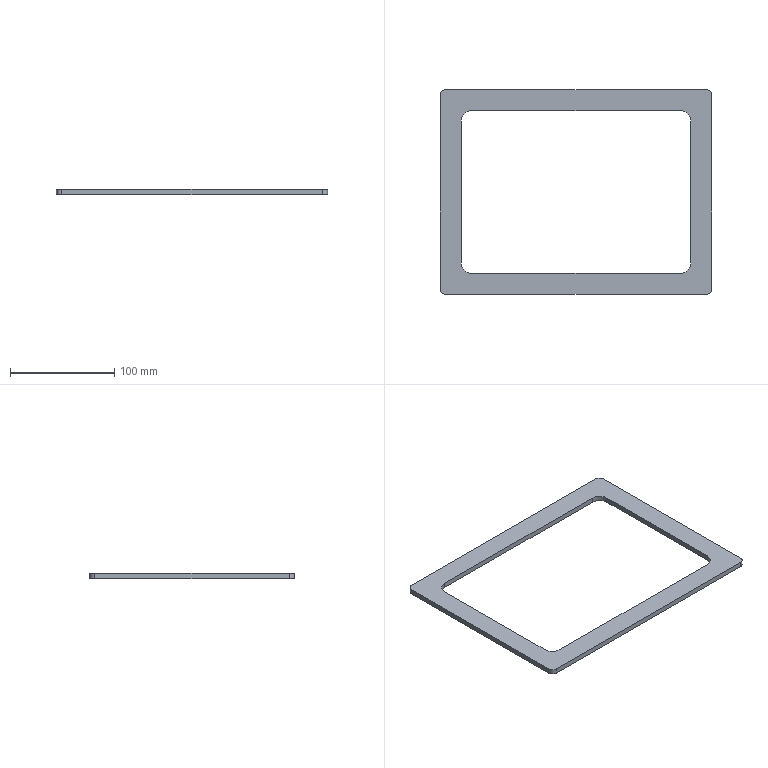Part | SolidWorks | features Fillet 2, Extrusion 1 | 1 solid | 18 faces | box 260 x 196 x 5 mm | volume 83522 mm3 | plane 10 | cylinder 8 | commonest cylinder face diameters 10 x4 20 x4
STEP:
#1=CARTESIAN_POINT('',(130.,-93.,5.));
#2=VERTEX_POINT('',#1);
#3=CARTESIAN_POINT('',(130.,93.,5.));
#4=VERTEX_POINT('',#3);
#5=CARTESIAN_POINT('',(130.,98.,5.));
#6=DIRECTION('',(0.,1.,0.));
#7=VECTOR('',#6,1000.);
#8=LINE('',#5,#7);
#9=EDGE_CURVE('',#2,#4,#8,.T.);
#10=ORIENTED_EDGE('',*,*,#9,.T.);
#11=CARTESIAN_POINT('',(125.,98.,5.));
#12=VERTEX_POINT('',#11);
#13=CARTESIAN_POINT('',(125.,93.,5.));
#14=DIRECTION('',(0.,0.,1.));
#15=DIRECTION('',(1.,0.,0.));
#16=AXIS2_PLACEMENT_3D('',#13,#14,#15);
#17=CIRCLE('',#16,5.);
#18=EDGE_CURVE('',#4,#12,#17,.T.);
#19=ORIENTED_EDGE('',*,*,#18,.T.);
#20=CARTESIAN_POINT('',(-125.,98.,5.));
#21=VERTEX_POINT('',#20);
#22=CARTESIAN_POINT('',(-130.,98.,5.));
#23=DIRECTION('',(-1.,0.,0.));
#24=VECTOR('',#23,1000.);
#25=LINE('',#22,#24);
#26=EDGE_CURVE('',#12,#21,#25,.T.);
#27=ORIENTED_EDGE('',*,*,#26,.T.);
#28=CARTESIAN_POINT('',(-130.,93.,5.));
#29=VERTEX_POINT('',#28);
#30=CARTESIAN_POINT('',(-125.,93.,5.));
#31=DIRECTION('',(0.,0.,1.));
#32=DIRECTION('',(1.,0.,0.));
#33=AXIS2_PLACEMENT_3D('',#30,#31,#32);
#34=CIRCLE('',#33,5.);
#35=EDGE_CURVE('',#21,#29,#34,.T.);
#36=ORIENTED_EDGE('',*,*,#35,.T.);
#37=CARTESIAN_POINT('',(-130.,-93.,5.));
#38=VERTEX_POINT('',#37);
#39=CARTESIAN_POINT('',(-130.,98.,5.));
#40=DIRECTION('',(0.,-1.,0.));
#41=VECTOR('',#40,1000.);
#42=LINE('',#39,#41);
#43=EDGE_CURVE('',#29,#38,#42,.T.);
#44=ORIENTED_EDGE('',*,*,#43,.T.);
#45=CARTESIAN_POINT('',(-125.,-98.,5.));
#46=VERTEX_POINT('',#45);
#47=CARTESIAN_POINT('',(-125.,-93.,5.));
#48=DIRECTION('',(0.,0.,1.));
#49=DIRECTION('',(1.,0.,0.));
#50=AXIS2_PLACEMENT_3D('',#47,#48,#49);
#51=CIRCLE('',#50,5.);
#52=EDGE_CURVE('',#38,#46,#51,.T.);
#53=ORIENTED_EDGE('',*,*,#52,.T.);
#54=CARTESIAN_POINT('',(125.,-98.,5.));
#55=VERTEX_POINT('',#54);
#56=CARTESIAN_POINT('',(-130.,-98.,5.));
#57=DIRECTION('',(1.,0.,0.));
#58=VECTOR('',#57,1000.);
#59=LINE('',#56,#58);
#60=EDGE_CURVE('',#46,#55,#59,.T.);
#61=ORIENTED_EDGE('',*,*,#60,.T.);
#62=CARTESIAN_POINT('',(125.,-93.,5.));
#63=DIRECTION('',(0.,0.,1.));
#64=DIRECTION('',(1.,0.,0.));
#65=AXIS2_PLACEMENT_3D('',#62,#63,#64);
#66=CIRCLE('',#65,5.);
#67=EDGE_CURVE('',#55,#2,#66,.T.);
#68=ORIENTED_EDGE('',*,*,#67,.T.);
#69=EDGE_LOOP('',(#10,#19,#27,#36,#44,#53,#61,#68));
#70=FACE_OUTER_BOUND('',#69,.T.);
#71=CARTESIAN_POINT('',(-100.,-78.,5.));
#72=VERTEX_POINT('',#71);
#73=CARTESIAN_POINT('',(100.,-78.,5.));
#74=VERTEX_POINT('',#73);
#75=CARTESIAN_POINT('',(-110.,-78.,5.));
#76=DIRECTION('',(1.,0.,0.));
#77=VECTOR('',#76,1000.);
#78=LINE('',#75,#77);
#79=EDGE_CURVE('',#72,#74,#78,.T.);
#80=ORIENTED_EDGE('',*,*,#79,.F.);
#81=CARTESIAN_POINT('',(-110.,-68.,5.));
#82=VERTEX_POINT('',#81);
#83=CARTESIAN_POINT('',(-100.,-68.,5.));
#84=DIRECTION('',(0.,0.,-1.));
#85=DIRECTION('',(1.,0.,0.));
#86=AXIS2_PLACEMENT_3D('',#83,#84,#85);
#87=CIRCLE('',#86,10.);
#88=EDGE_CURVE('',#72,#82,#87,.T.);
#89=ORIENTED_EDGE('',*,*,#88,.T.);
#90=CARTESIAN_POINT('',(-110.,68.,5.));
#91=VERTEX_POINT('',#90);
#92=CARTESIAN_POINT('',(-110.,78.,5.));
#93=DIRECTION('',(0.,-1.,0.));
#94=VECTOR('',#93,1000.);
#95=LINE('',#92,#94);
#96=EDGE_CURVE('',#91,#82,#95,.T.);
#97=ORIENTED_EDGE('',*,*,#96,.F.);
#98=CARTESIAN_POINT('',(-100.,78.,5.));
#99=VERTEX_POINT('',#98);
#100=CARTESIAN_POINT('',(-100.,68.,5.));
#101=DIRECTION('',(0.,0.,-1.));
#102=DIRECTION('',(1.,0.,0.));
#103=AXIS2_PLACEMENT_3D('',#100,#101,#102);
#104=CIRCLE('',#103,10.);
#105=EDGE_CURVE('',#91,#99,#104,.T.);
#106=ORIENTED_EDGE('',*,*,#105,.T.);
#107=CARTESIAN_POINT('',(100.,78.,5.));
#108=VERTEX_POINT('',#107);
#109=CARTESIAN_POINT('',(-110.,78.,5.));
#110=DIRECTION('',(-1.,0.,0.));
#111=VECTOR('',#110,1000.);
#112=LINE('',#109,#111);
#113=EDGE_CURVE('',#108,#99,#112,.T.);
#114=ORIENTED_EDGE('',*,*,#113,.F.);
#115=CARTESIAN_POINT('',(110.,68.,5.));
#116=VERTEX_POINT('',#115);
#117=CARTESIAN_POINT('',(100.,68.,5.));
#118=DIRECTION('',(0.,0.,-1.));
#119=DIRECTION('',(1.,0.,0.));
#120=AXIS2_PLACEMENT_3D('',#117,#118,#119);
#121=CIRCLE('',#120,10.);
#122=EDGE_CURVE('',#108,#116,#121,.T.);
#123=ORIENTED_EDGE('',*,*,#122,.T.);
#124=CARTESIAN_POINT('',(110.,-68.,5.));
#125=VERTEX_POINT('',#124);
#126=CARTESIAN_POINT('',(110.,78.,5.));
#127=DIRECTION('',(0.,1.,0.));
#128=VECTOR('',#127,1000.);
#129=LINE('',#126,#128);
#130=EDGE_CURVE('',#125,#116,#129,.T.);
#131=ORIENTED_EDGE('',*,*,#130,.F.);
#132=CARTESIAN_POINT('',(100.,-68.,5.));
#133=DIRECTION('',(0.,0.,-1.));
#134=DIRECTION('',(1.,0.,0.));
#135=AXIS2_PLACEMENT_3D('',#132,#133,#134);
#136=CIRCLE('',#135,10.);
#137=EDGE_CURVE('',#125,#74,#136,.T.);
#138=ORIENTED_EDGE('',*,*,#137,.T.);
#139=EDGE_LOOP('',(#80,#89,#97,#106,#114,#123,#131,#138));
#140=FACE_BOUND('',#139,.T.);
#141=CARTESIAN_POINT('',(0.,0.,5.));
#142=DIRECTION('',(0.,0.,1.));
#143=DIRECTION('',(1.,0.,0.));
#144=AXIS2_PLACEMENT_3D('',#141,#142,#143);
#145=PLANE('',#144);
#146=ADVANCED_FACE('',(#70,#140),#145,.T.);
#147=CARTESIAN_POINT('',(125.,98.,0.));
#148=VERTEX_POINT('',#147);
#149=CARTESIAN_POINT('',(-125.,98.,0.));
#150=VERTEX_POINT('',#149);
#151=CARTESIAN_POINT('',(-130.,98.,0.));
#152=DIRECTION('',(-1.,0.,0.));
#153=VECTOR('',#152,1000.);
#154=LINE('',#151,#153);
#155=EDGE_CURVE('',#148,#150,#154,.T.);
#156=ORIENTED_EDGE('',*,*,#155,.F.);
#157=CARTESIAN_POINT('',(130.,93.,0.));
#158=VERTEX_POINT('',#157);
#159=CARTESIAN_POINT('',(125.,93.,0.));
#160=DIRECTION('',(0.,0.,-1.));
#161=DIRECTION('',(1.,0.,0.));
#162=AXIS2_PLACEMENT_3D('',#159,#160,#161);
#163=CIRCLE('',#162,5.);
#164=EDGE_CURVE('',#148,#158,#163,.T.);
#165=ORIENTED_EDGE('',*,*,#164,.T.);
#166=CARTESIAN_POINT('',(130.,-93.,0.));
#167=VERTEX_POINT('',#166);
#168=CARTESIAN_POINT('',(130.,98.,0.));
#169=DIRECTION('',(0.,1.,0.));
#170=VECTOR('',#169,1000.);
#171=LINE('',#168,#170);
#172=EDGE_CURVE('',#167,#158,#171,.T.);
#173=ORIENTED_EDGE('',*,*,#172,.F.);
#174=CARTESIAN_POINT('',(125.,-98.,0.));
#175=VERTEX_POINT('',#174);
#176=CARTESIAN_POINT('',(125.,-93.,0.));
#177=DIRECTION('',(0.,0.,-1.));
#178=DIRECTION('',(1.,0.,0.));
#179=AXIS2_PLACEMENT_3D('',#176,#177,#178);
#180=CIRCLE('',#179,5.);
#181=EDGE_CURVE('',#167,#175,#180,.T.);
#182=ORIENTED_EDGE('',*,*,#181,.T.);
#183=CARTESIAN_POINT('',(-125.,-98.,0.));
#184=VERTEX_POINT('',#183);
#185=CARTESIAN_POINT('',(-130.,-98.,0.));
#186=DIRECTION('',(1.,0.,0.));
#187=VECTOR('',#186,1000.);
#188=LINE('',#185,#187);
#189=EDGE_CURVE('',#184,#175,#188,.T.);
#190=ORIENTED_EDGE('',*,*,#189,.F.);
#191=CARTESIAN_POINT('',(-130.,-93.,0.));
#192=VERTEX_POINT('',#191);
#193=CARTESIAN_POINT('',(-125.,-93.,0.));
#194=DIRECTION('',(0.,0.,-1.));
#195=DIRECTION('',(1.,0.,0.));
#196=AXIS2_PLACEMENT_3D('',#193,#194,#195);
#197=CIRCLE('',#196,5.);
#198=EDGE_CURVE('',#184,#192,#197,.T.);
#199=ORIENTED_EDGE('',*,*,#198,.T.);
#200=CARTESIAN_POINT('',(-130.,93.,0.));
#201=VERTEX_POINT('',#200);
#202=CARTESIAN_POINT('',(-130.,98.,0.));
#203=DIRECTION('',(0.,-1.,0.));
#204=VECTOR('',#203,1000.);
#205=LINE('',#202,#204);
#206=EDGE_CURVE('',#201,#192,#205,.T.);
#207=ORIENTED_EDGE('',*,*,#206,.F.);
#208=CARTESIAN_POINT('',(-125.,93.,0.));
#209=DIRECTION('',(0.,0.,-1.));
#210=DIRECTION('',(1.,0.,0.));
#211=AXIS2_PLACEMENT_3D('',#208,#209,#210);
#212=CIRCLE('',#211,5.);
#213=EDGE_CURVE('',#201,#150,#212,.T.);
#214=ORIENTED_EDGE('',*,*,#213,.T.);
#215=EDGE_LOOP('',(#156,#165,#173,#182,#190,#199,#207,#214));
#216=FACE_OUTER_BOUND('',#215,.T.);
#217=CARTESIAN_POINT('',(100.,78.,0.));
#218=VERTEX_POINT('',#217);
#219=CARTESIAN_POINT('',(-100.,78.,0.));
#220=VERTEX_POINT('',#219);
#221=CARTESIAN_POINT('',(-110.,78.,0.));
#222=DIRECTION('',(-1.,0.,0.));
#223=VECTOR('',#222,1000.);
#224=LINE('',#221,#223);
#225=EDGE_CURVE('',#218,#220,#224,.T.);
#226=ORIENTED_EDGE('',*,*,#225,.T.);
#227=CARTESIAN_POINT('',(-110.,68.,0.));
#228=VERTEX_POINT('',#227);
#229=CARTESIAN_POINT('',(-100.,68.,0.));
#230=DIRECTION('',(0.,0.,1.));
#231=DIRECTION('',(1.,0.,0.));
#232=AXIS2_PLACEMENT_3D('',#229,#230,#231);
#233=CIRCLE('',#232,10.);
#234=EDGE_CURVE('',#220,#228,#233,.T.);
#235=ORIENTED_EDGE('',*,*,#234,.T.);
#236=CARTESIAN_POINT('',(-110.,-68.,0.));
#237=VERTEX_POINT('',#236);
#238=CARTESIAN_POINT('',(-110.,78.,0.));
#239=DIRECTION('',(0.,-1.,0.));
#240=VECTOR('',#239,1000.);
#241=LINE('',#238,#240);
#242=EDGE_CURVE('',#228,#237,#241,.T.);
#243=ORIENTED_EDGE('',*,*,#242,.T.);
#244=CARTESIAN_POINT('',(-100.,-78.,0.));
#245=VERTEX_POINT('',#244);
#246=CARTESIAN_POINT('',(-100.,-68.,0.));
#247=DIRECTION('',(0.,0.,1.));
#248=DIRECTION('',(1.,0.,0.));
#249=AXIS2_PLACEMENT_3D('',#246,#247,#248);
#250=CIRCLE('',#249,10.);
#251=EDGE_CURVE('',#237,#245,#250,.T.);
#252=ORIENTED_EDGE('',*,*,#251,.T.);
#253=CARTESIAN_POINT('',(100.,-78.,0.));
#254=VERTEX_POINT('',#253);
#255=CARTESIAN_POINT('',(-110.,-78.,0.));
#256=DIRECTION('',(1.,0.,0.));
#257=VECTOR('',#256,1000.);
#258=LINE('',#255,#257);
#259=EDGE_CURVE('',#245,#254,#258,.T.);
#260=ORIENTED_EDGE('',*,*,#259,.T.);
#261=CARTESIAN_POINT('',(110.,-68.,0.));
#262=VERTEX_POINT('',#261);
#263=CARTESIAN_POINT('',(100.,-68.,0.));
#264=DIRECTION('',(0.,0.,1.));
#265=DIRECTION('',(1.,0.,0.));
#266=AXIS2_PLACEMENT_3D('',#263,#264,#265);
#267=CIRCLE('',#266,10.);
#268=EDGE_CURVE('',#254,#262,#267,.T.);
#269=ORIENTED_EDGE('',*,*,#268,.T.);
#270=CARTESIAN_POINT('',(110.,68.,0.));
#271=VERTEX_POINT('',#270);
#272=CARTESIAN_POINT('',(110.,78.,0.));
#273=DIRECTION('',(0.,1.,0.));
#274=VECTOR('',#273,1000.);
#275=LINE('',#272,#274);
#276=EDGE_CURVE('',#262,#271,#275,.T.);
#277=ORIENTED_EDGE('',*,*,#276,.T.);
#278=CARTESIAN_POINT('',(100.,68.,0.));
#279=DIRECTION('',(0.,0.,1.));
#280=DIRECTION('',(1.,0.,0.));
#281=AXIS2_PLACEMENT_3D('',#278,#279,#280);
#282=CIRCLE('',#281,10.);
#283=EDGE_CURVE('',#271,#218,#282,.T.);
#284=ORIENTED_EDGE('',*,*,#283,.T.);
#285=EDGE_LOOP('',(#226,#235,#243,#252,#260,#269,#277,#284));
#286=FACE_BOUND('',#285,.T.);
#287=CARTESIAN_POINT('',(0.,0.,0.));
#288=DIRECTION('',(0.,0.,1.));
#289=DIRECTION('',(1.,0.,0.));
#290=AXIS2_PLACEMENT_3D('',#287,#288,#289);
#291=PLANE('',#290);
#292=ADVANCED_FACE('',(#216,#286),#291,.F.);
#293=ORIENTED_EDGE('',*,*,#206,.T.);
#294=CARTESIAN_POINT('',(-130.,-93.,5.));
#295=DIRECTION('',(0.,0.,1.));
#296=VECTOR('',#295,1000.);
#297=LINE('',#294,#296);
#298=EDGE_CURVE('',#192,#38,#297,.T.);
#299=ORIENTED_EDGE('',*,*,#298,.T.);
#300=ORIENTED_EDGE('',*,*,#43,.F.);
#301=CARTESIAN_POINT('',(-130.,93.,5.));
#302=DIRECTION('',(0.,0.,-1.));
#303=VECTOR('',#302,1000.);
#304=LINE('',#301,#303);
#305=EDGE_CURVE('',#29,#201,#304,.T.);
#306=ORIENTED_EDGE('',*,*,#305,.T.);
#307=EDGE_LOOP('',(#293,#299,#300,#306));
#308=FACE_OUTER_BOUND('',#307,.T.);
#309=CARTESIAN_POINT('',(-130.,98.,5.));
#310=DIRECTION('',(1.,0.,0.));
#311=DIRECTION('',(0.,0.,-1.));
#312=AXIS2_PLACEMENT_3D('',#309,#310,#311);
#313=PLANE('',#312);
#314=ADVANCED_FACE('',(#308),#313,.F.);
#315=ORIENTED_EDGE('',*,*,#189,.T.);
#316=CARTESIAN_POINT('',(125.,-98.,5.));
#317=DIRECTION('',(0.,0.,1.));
#318=VECTOR('',#317,1000.);
#319=LINE('',#316,#318);
#320=EDGE_CURVE('',#175,#55,#319,.T.);
#321=ORIENTED_EDGE('',*,*,#320,.T.);
#322=ORIENTED_EDGE('',*,*,#60,.F.);
#323=CARTESIAN_POINT('',(-125.,-98.,5.));
#324=DIRECTION('',(0.,0.,-1.));
#325=VECTOR('',#324,1000.);
#326=LINE('',#323,#325);
#327=EDGE_CURVE('',#46,#184,#326,.T.);
#328=ORIENTED_EDGE('',*,*,#327,.T.);
#329=EDGE_LOOP('',(#315,#321,#322,#328));
#330=FACE_OUTER_BOUND('',#329,.T.);
#331=CARTESIAN_POINT('',(-130.,-98.,5.));
#332=DIRECTION('',(0.,1.,0.));
#333=DIRECTION('',(0.,0.,1.));
#334=AXIS2_PLACEMENT_3D('',#331,#332,#333);
#335=PLANE('',#334);
#336=ADVANCED_FACE('',(#330),#335,.F.);
#337=ORIENTED_EDGE('',*,*,#172,.T.);
#338=CARTESIAN_POINT('',(130.,93.,5.));
#339=DIRECTION('',(0.,0.,1.));
#340=VECTOR('',#339,1000.);
#341=LINE('',#338,#340);
#342=EDGE_CURVE('',#158,#4,#341,.T.);
#343=ORIENTED_EDGE('',*,*,#342,.T.);
#344=ORIENTED_EDGE('',*,*,#9,.F.);
#345=CARTESIAN_POINT('',(130.,-93.,5.));
#346=DIRECTION('',(0.,0.,-1.));
#347=VECTOR('',#346,1000.);
#348=LINE('',#345,#347);
#349=EDGE_CURVE('',#2,#167,#348,.T.);
#350=ORIENTED_EDGE('',*,*,#349,.T.);
#351=EDGE_LOOP('',(#337,#343,#344,#350));
#352=FACE_OUTER_BOUND('',#351,.T.);
#353=CARTESIAN_POINT('',(130.,98.,5.));
#354=DIRECTION('',(-1.,0.,0.));
#355=DIRECTION('',(0.,0.,1.));
#356=AXIS2_PLACEMENT_3D('',#353,#354,#355);
#357=PLANE('',#356);
#358=ADVANCED_FACE('',(#352),#357,.F.);
#359=ORIENTED_EDGE('',*,*,#26,.F.);
#360=CARTESIAN_POINT('',(125.,98.,5.));
#361=DIRECTION('',(0.,0.,-1.));
#362=VECTOR('',#361,1000.);
#363=LINE('',#360,#362);
#364=EDGE_CURVE('',#12,#148,#363,.T.);
#365=ORIENTED_EDGE('',*,*,#364,.T.);
#366=ORIENTED_EDGE('',*,*,#155,.T.);
#367=CARTESIAN_POINT('',(-125.,98.,5.));
#368=DIRECTION('',(0.,0.,1.));
#369=VECTOR('',#368,1000.);
#370=LINE('',#367,#369);
#371=EDGE_CURVE('',#150,#21,#370,.T.);
#372=ORIENTED_EDGE('',*,*,#371,.T.);
#373=EDGE_LOOP('',(#359,#365,#366,#372));
#374=FACE_OUTER_BOUND('',#373,.T.);
#375=CARTESIAN_POINT('',(-130.,98.,5.));
#376=DIRECTION('',(0.,-1.,0.));
#377=DIRECTION('',(0.,0.,-1.));
#378=AXIS2_PLACEMENT_3D('',#375,#376,#377);
#379=PLANE('',#378);
#380=ADVANCED_FACE('',(#374),#379,.F.);
#381=ORIENTED_EDGE('',*,*,#242,.F.);
#382=CARTESIAN_POINT('',(-110.,68.,5.));
#383=DIRECTION('',(0.,0.,1.));
#384=VECTOR('',#383,1000.);
#385=LINE('',#382,#384);
#386=EDGE_CURVE('',#228,#91,#385,.T.);
#387=ORIENTED_EDGE('',*,*,#386,.T.);
#388=ORIENTED_EDGE('',*,*,#96,.T.);
#389=CARTESIAN_POINT('',(-110.,-68.,0.));
#390=DIRECTION('',(0.,0.,-1.));
#391=VECTOR('',#390,1000.);
#392=LINE('',#389,#391);
#393=EDGE_CURVE('',#82,#237,#392,.T.);
#394=ORIENTED_EDGE('',*,*,#393,.T.);
#395=EDGE_LOOP('',(#381,#387,#388,#394));
#396=FACE_OUTER_BOUND('',#395,.T.);
#397=CARTESIAN_POINT('',(-110.,78.,5.));
#398=DIRECTION('',(1.,0.,0.));
#399=DIRECTION('',(0.,1.,0.));
#400=AXIS2_PLACEMENT_3D('',#397,#398,#399);
#401=PLANE('',#400);
#402=ADVANCED_FACE('',(#396),#401,.T.);
#403=ORIENTED_EDGE('',*,*,#259,.F.);
#404=CARTESIAN_POINT('',(-100.,-78.,5.));
#405=DIRECTION('',(0.,0.,1.));
#406=VECTOR('',#405,1000.);
#407=LINE('',#404,#406);
#408=EDGE_CURVE('',#245,#72,#407,.T.);
#409=ORIENTED_EDGE('',*,*,#408,.T.);
#410=ORIENTED_EDGE('',*,*,#79,.T.);
#411=CARTESIAN_POINT('',(100.,-78.,0.));
#412=DIRECTION('',(0.,0.,-1.));
#413=VECTOR('',#412,1000.);
#414=LINE('',#411,#413);
#415=EDGE_CURVE('',#74,#254,#414,.T.);
#416=ORIENTED_EDGE('',*,*,#415,.T.);
#417=EDGE_LOOP('',(#403,#409,#410,#416));
#418=FACE_OUTER_BOUND('',#417,.T.);
#419=CARTESIAN_POINT('',(-110.,-78.,5.));
#420=DIRECTION('',(0.,1.,0.));
#421=DIRECTION('',(-1.,0.,0.));
#422=AXIS2_PLACEMENT_3D('',#419,#420,#421);
#423=PLANE('',#422);
#424=ADVANCED_FACE('',(#418),#423,.T.);
#425=ORIENTED_EDGE('',*,*,#130,.T.);
#426=CARTESIAN_POINT('',(110.,68.,0.));
#427=DIRECTION('',(0.,0.,-1.));
#428=VECTOR('',#427,1000.);
#429=LINE('',#426,#428);
#430=EDGE_CURVE('',#116,#271,#429,.T.);
#431=ORIENTED_EDGE('',*,*,#430,.T.);
#432=ORIENTED_EDGE('',*,*,#276,.F.);
#433=CARTESIAN_POINT('',(110.,-68.,5.));
#434=DIRECTION('',(0.,0.,1.));
#435=VECTOR('',#434,1000.);
#436=LINE('',#433,#435);
#437=EDGE_CURVE('',#262,#125,#436,.T.);
#438=ORIENTED_EDGE('',*,*,#437,.T.);
#439=EDGE_LOOP('',(#425,#431,#432,#438));
#440=FACE_OUTER_BOUND('',#439,.T.);
#441=CARTESIAN_POINT('',(110.,78.,5.));
#442=DIRECTION('',(-1.,0.,0.));
#443=DIRECTION('',(0.,-1.,0.));
#444=AXIS2_PLACEMENT_3D('',#441,#442,#443);
#445=PLANE('',#444);
#446=ADVANCED_FACE('',(#440),#445,.T.);
#447=ORIENTED_EDGE('',*,*,#225,.F.);
#448=CARTESIAN_POINT('',(100.,78.,5.));
#449=DIRECTION('',(0.,0.,1.));
#450=VECTOR('',#449,1000.);
#451=LINE('',#448,#450);
#452=EDGE_CURVE('',#218,#108,#451,.T.);
#453=ORIENTED_EDGE('',*,*,#452,.T.);
#454=ORIENTED_EDGE('',*,*,#113,.T.);
#455=CARTESIAN_POINT('',(-100.,78.,0.));
#456=DIRECTION('',(0.,0.,-1.));
#457=VECTOR('',#456,1000.);
#458=LINE('',#455,#457);
#459=EDGE_CURVE('',#99,#220,#458,.T.);
#460=ORIENTED_EDGE('',*,*,#459,.T.);
#461=EDGE_LOOP('',(#447,#453,#454,#460));
#462=FACE_OUTER_BOUND('',#461,.T.);
#463=CARTESIAN_POINT('',(-110.,78.,5.));
#464=DIRECTION('',(0.,-1.,0.));
#465=DIRECTION('',(0.,0.,-1.));
#466=AXIS2_PLACEMENT_3D('',#463,#464,#465);
#467=PLANE('',#466);
#468=ADVANCED_FACE('',(#462),#467,.T.);
#469=ORIENTED_EDGE('',*,*,#18,.F.);
#470=ORIENTED_EDGE('',*,*,#342,.F.);
#471=ORIENTED_EDGE('',*,*,#164,.F.);
#472=ORIENTED_EDGE('',*,*,#364,.F.);
#473=EDGE_LOOP('',(#469,#470,#471,#472));
#474=FACE_OUTER_BOUND('',#473,.T.);
#475=CARTESIAN_POINT('',(125.,93.,5.));
#476=DIRECTION('',(0.,0.,-1.));
#477=DIRECTION('',(-1.,0.,0.));
#478=AXIS2_PLACEMENT_3D('',#475,#476,#477);
#479=CYLINDRICAL_SURFACE('',#478,5.);
#480=ADVANCED_FACE('',(#474),#479,.T.);
#481=ORIENTED_EDGE('',*,*,#67,.F.);
#482=ORIENTED_EDGE('',*,*,#320,.F.);
#483=ORIENTED_EDGE('',*,*,#181,.F.);
#484=ORIENTED_EDGE('',*,*,#349,.F.);
#485=EDGE_LOOP('',(#481,#482,#483,#484));
#486=FACE_OUTER_BOUND('',#485,.T.);
#487=CARTESIAN_POINT('',(125.,-93.,5.));
#488=DIRECTION('',(0.,0.,-1.));
#489=DIRECTION('',(-1.,0.,0.));
#490=AXIS2_PLACEMENT_3D('',#487,#488,#489);
#491=CYLINDRICAL_SURFACE('',#490,5.);
#492=ADVANCED_FACE('',(#486),#491,.T.);
#493=ORIENTED_EDGE('',*,*,#52,.F.);
#494=ORIENTED_EDGE('',*,*,#298,.F.);
#495=ORIENTED_EDGE('',*,*,#198,.F.);
#496=ORIENTED_EDGE('',*,*,#327,.F.);
#497=EDGE_LOOP('',(#493,#494,#495,#496));
#498=FACE_OUTER_BOUND('',#497,.T.);
#499=CARTESIAN_POINT('',(-125.,-93.,5.));
#500=DIRECTION('',(0.,0.,-1.));
#501=DIRECTION('',(-1.,0.,0.));
#502=AXIS2_PLACEMENT_3D('',#499,#500,#501);
#503=CYLINDRICAL_SURFACE('',#502,5.);
#504=ADVANCED_FACE('',(#498),#503,.T.);
#505=ORIENTED_EDGE('',*,*,#35,.F.);
#506=ORIENTED_EDGE('',*,*,#371,.F.);
#507=ORIENTED_EDGE('',*,*,#213,.F.);
#508=ORIENTED_EDGE('',*,*,#305,.F.);
#509=EDGE_LOOP('',(#505,#506,#507,#508));
#510=FACE_OUTER_BOUND('',#509,.T.);
#511=CARTESIAN_POINT('',(-125.,93.,5.));
#512=DIRECTION('',(0.,0.,-1.));
#513=DIRECTION('',(-1.,0.,0.));
#514=AXIS2_PLACEMENT_3D('',#511,#512,#513);
#515=CYLINDRICAL_SURFACE('',#514,5.);
#516=ADVANCED_FACE('',(#510),#515,.T.);
#517=ORIENTED_EDGE('',*,*,#122,.F.);
#518=ORIENTED_EDGE('',*,*,#452,.F.);
#519=ORIENTED_EDGE('',*,*,#283,.F.);
#520=ORIENTED_EDGE('',*,*,#430,.F.);
#521=EDGE_LOOP('',(#517,#518,#519,#520));
#522=FACE_OUTER_BOUND('',#521,.T.);
#523=CARTESIAN_POINT('',(100.,68.,5.));
#524=DIRECTION('',(0.,0.,1.));
#525=DIRECTION('',(1.,0.,0.));
#526=AXIS2_PLACEMENT_3D('',#523,#524,#525);
#527=CYLINDRICAL_SURFACE('',#526,10.);
#528=ADVANCED_FACE('',(#522),#527,.F.);
#529=ORIENTED_EDGE('',*,*,#105,.F.);
#530=ORIENTED_EDGE('',*,*,#386,.F.);
#531=ORIENTED_EDGE('',*,*,#234,.F.);
#532=ORIENTED_EDGE('',*,*,#459,.F.);
#533=EDGE_LOOP('',(#529,#530,#531,#532));
#534=FACE_OUTER_BOUND('',#533,.T.);
#535=CARTESIAN_POINT('',(-100.,68.,5.));
#536=DIRECTION('',(0.,0.,1.));
#537=DIRECTION('',(1.,0.,0.));
#538=AXIS2_PLACEMENT_3D('',#535,#536,#537);
#539=CYLINDRICAL_SURFACE('',#538,10.);
#540=ADVANCED_FACE('',(#534),#539,.F.);
#541=ORIENTED_EDGE('',*,*,#88,.F.);
#542=ORIENTED_EDGE('',*,*,#408,.F.);
#543=ORIENTED_EDGE('',*,*,#251,.F.);
#544=ORIENTED_EDGE('',*,*,#393,.F.);
#545=EDGE_LOOP('',(#541,#542,#543,#544));
#546=FACE_OUTER_BOUND('',#545,.T.);
#547=CARTESIAN_POINT('',(-100.,-68.,5.));
#548=DIRECTION('',(0.,0.,1.));
#549=DIRECTION('',(1.,0.,0.));
#550=AXIS2_PLACEMENT_3D('',#547,#548,#549);
#551=CYLINDRICAL_SURFACE('',#550,10.);
#552=ADVANCED_FACE('',(#546),#551,.F.);
#553=ORIENTED_EDGE('',*,*,#137,.F.);
#554=ORIENTED_EDGE('',*,*,#437,.F.);
#555=ORIENTED_EDGE('',*,*,#268,.F.);
#556=ORIENTED_EDGE('',*,*,#415,.F.);
#557=EDGE_LOOP('',(#553,#554,#555,#556));
#558=FACE_OUTER_BOUND('',#557,.T.);
#559=CARTESIAN_POINT('',(100.,-68.,5.));
#560=DIRECTION('',(0.,0.,1.));
#561=DIRECTION('',(1.,0.,0.));
#562=AXIS2_PLACEMENT_3D('',#559,#560,#561);
#563=CYLINDRICAL_SURFACE('',#562,10.);
#564=ADVANCED_FACE('',(#558),#563,.F.);
#565=CLOSED_SHELL('',(#146,#292,#314,#336,#358,#380,#402,#424,#446,#468,#480,#492,#504,#516,#528,#540,#552,#564));
#566=MANIFOLD_SOLID_BREP('',#565);
#567=CARTESIAN_POINT('',(0.,0.,0.));
#568=DIRECTION('',(0.,0.,1.));
#569=DIRECTION('',(1.,0.,0.));
#570=AXIS2_PLACEMENT_3D('',#567,#568,#569);
#571=(LENGTH_UNIT()NAMED_UNIT(*)SI_UNIT(.MILLI.,.METRE.));
#572=UNCERTAINTY_MEASURE_WITH_UNIT(LENGTH_MEASURE(0.00001),#571,'','');
#573=(NAMED_UNIT(*)PLANE_ANGLE_UNIT()SI_UNIT($,.RADIAN.));
#574=(NAMED_UNIT(*)SI_UNIT($,.STERADIAN.)SOLID_ANGLE_UNIT());
#575=(GEOMETRIC_REPRESENTATION_CONTEXT(3)GLOBAL_UNCERTAINTY_ASSIGNED_CONTEXT((#572))GLOBAL_UNIT_ASSIGNED_CONTEXT((#571,#573,#574))REPRESENTATION_CONTEXT('',''));
#576=ADVANCED_BREP_SHAPE_REPRESENTATION('',(#566,#570),#575);